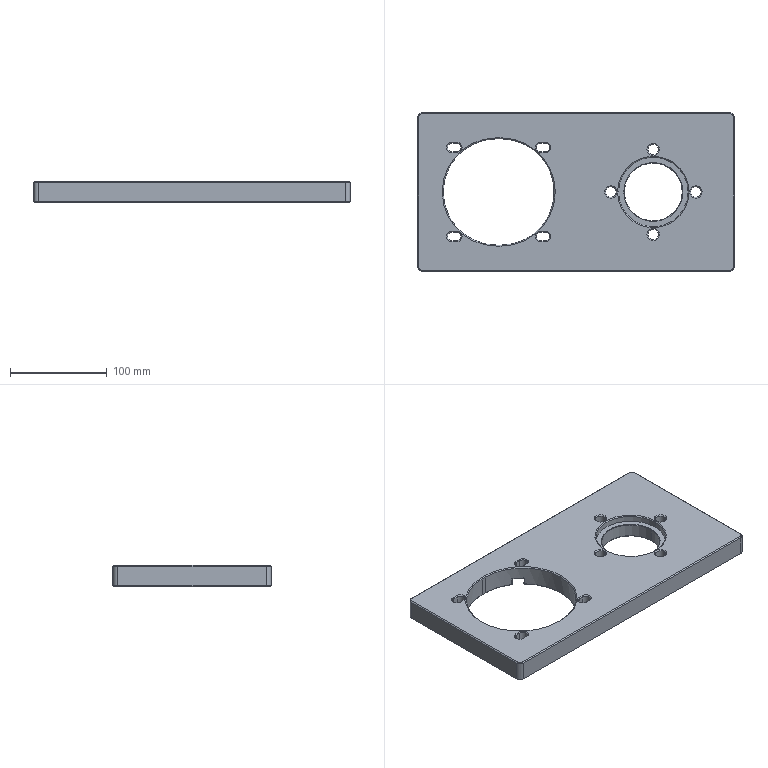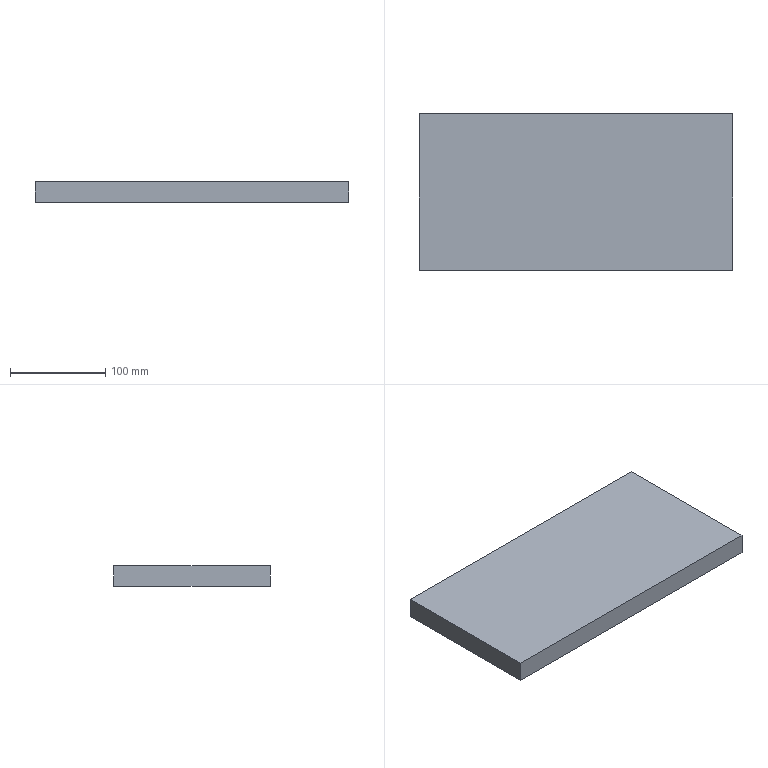CAM job | NX | 3-axis milling, drilling | part box 328 x 164 x 22 mm | stock box 328 x 164 x 22 mm
Tools:
number,name,description,diameter,corner_radius,flute_length,length,flutes
1,ZXZ,Milling Tool-5 Parameters,6.0,0.0,50.0,75.0,2
11,11.0ZT,Drilling Tool,11.0,0.0,35.0,50.0,2
16,6.8ZT,Drilling Tool,6.8,0.0,35.0,50.0,2
10,D10C,Milling Tool-5 Parameters,10.0,0.0,50.0,75.0,2
9,D10JING,Milling Tool-5 Parameters,10.0,0.0,50.0,75.0,2
6,D6,Milling Tool-5 Parameters,6.0,0.0,50.0,75.0,2
7,D10A45,Milling Tool-5 Parameters,10.0,0.0,50.0,75.0,2
13,3.3ZT,Drilling Tool,3.3,0.0,35.0,50.0,2
5,D3R0.5,Milling Tool-5 Parameters,3.0,0.5,50.0,75.0,2
2,D26,Milling Tool-5 Parameters,26.0,0.0,50.0,75.0,2
Operations:
program,operation,operation_type,tool,method,geometry_group,spindle_rpm,surface_speed,feed_per_tooth,feed_cut,feed_plunge,cut_length_mm,path_length_mm,cut_time_min,machine_time_min
1,DRILLING,Operation,ZXZ,METHOD,A,5000.0,94.0,0.025,250.0,0.0,20.0,324.8,0.08,0.1105
1,DRILLING_COPY,Operation,ZXZ,METHOD,A,5000.0,94.0,0.025,250.0,0.0,16.0,376.918,0.064,0.1001
1,DRILLING_COPY_COPY,Operation,11.0ZT,METHOD,A,1200.0,41.0,0.1042,250.0,0.0,141.524,567.847,0.5661,0.6087
1,DRILLING_COPY_COPY_1,Operation,6.8ZT,METHOD,A,2000.0,42.0,0.0625,250.0,0.0,108.172,561.262,0.4327,0.478
1,HOLE_MILLING_COPY,CylinderMilling,D26,METHOD,A,1700.0,138.0,0.5882,2000.0,1000.0,5706.962,5780.962,2.88,2.888
1,HOLE_MILLING_COPY_COPY,CylinderMilling,D26,METHOD,A,1700.0,138.0,0.5882,2000.0,1000.0,8866.822,8972.422,4.453,4.464
1,HOLE_MILLING_COPY_COPY_COPY,CylinderMilling,D26,METHOD,A,1700.0,138.0,0.5882,2000.0,1000.0,47660.025,47806.225,23.912,23.927
1,ZLEVEL_PROFILE,ZLevelMilling,D10C,METHOD,A,3000.0,94.0,0.4167,2500.0,1000.0,10074.669,11142.386,4.458,4.565
1,ZLEVEL_PROFILE_COPY,ZLevelMilling,D10JING,METHOD,A,5000.0,157.0,0.1,1000.0,1000.0,97.808,1114.401,0.0978,0.1995
1,ZLEVEL_PROFILE_COPY_COPY,ZLevelMilling,D10JING,METHOD,A,5000.0,157.0,0.1,1000.0,1000.0,162.414,264.414,0.1624,0.1726
1,ZLEVEL_PROFILE_1,ZLevelMilling,D6,METHOD,A,4500.0,84.0,0.1778,1600.0,100.0,17199.194,17785.132,10.749,10.808
1,PLANAR_MILL_1,PlanarMilling,D10A45,METHOD,A,7500.0,141.0,0.0833,1250.0,100.0,1892.313,3214.008,1.514,1.646
1,PLANAR_MILL_1_COPY,PlanarMilling,D10A45,METHOD,A,7500.0,141.0,0.0833,1250.0,100.0,188.422,260.022,0.1507,0.1579
1,刀补9,ZLevelMilling,D10JING,METHOD,A,5000.0,157.0,0.1,1000.0,1000.0,329.294,431.294,0.3293,0.3395
1,刀补6,ZLevelMilling,D6,METHOD,A,5000.0,157.0,0.1,1000.0,1000.0,211.198,283.198,0.2112,0.2184
2,DRILLING_COPY_1,Operation,ZXZ,METHOD,B,5000.0,94.0,0.025,250.0,0.0,16.0,712.075,0.064,0.1336
2,DRILLING_COPY_COPY_1_COPY,Operation,3.3ZT,METHOD,B,2000.0,20.0,0.03,120.0,0.0,69.966,820.006,0.583,0.6581
2,HOLE_MILLING,CylinderMilling,D10C,METHOD,B,3500.0,109.0,0.3571,2500.0,1000.0,6418.096,6890.772,2.582,2.63
2,ZLEVEL_PROFILE_COPY_1,ZLevelMilling,D10C,METHOD,B,3000.0,94.0,0.4167,2500.0,1000.0,8437.032,11005.498,3.522,3.779
2,ZLEVEL_PROFILE_COPY_1_COPY,ZLevelMilling,D10JING,METHOD,B,5000.0,157.0,0.12,1200.0,1000.0,222.269,770.938,0.1863,0.2412
2,HOLE_MILLING_COPY_1,CylinderMilling,D10JING,METHOD,B,5000.0,157.0,0.12,1200.0,1000.0,778.654,1251.33,0.6529,0.7001
2,ZLEVEL_PROFILE_1_COPY,ZLevelMilling,D3R0.5,METHOD,B,7000.0,65.0,0.1786,2500.0,100.0,5602.218,6180.168,2.241,2.299
2,DRILLING_COPY_1_COPY,Operation,D10A45,METHOD,B,5000.0,94.0,0.025,250.0,0.0,22.6,725.275,0.0904,0.1607
2,PLANAR_MILL_1_COPY_1,PlanarMilling,D10A45,METHOD,B,7500.0,141.0,0.0833,1250.0,100.0,1938.816,2693.671,1.551,1.627